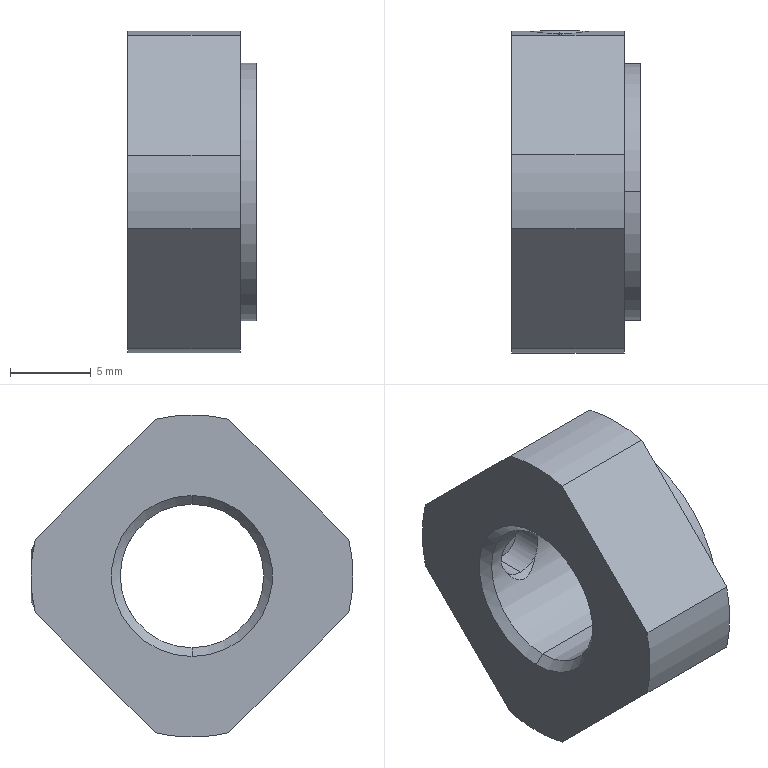Part | STEP file | Mirror BNR10 | 2 solids | 49 faces | box 8 x 20 x 20 mm | volume 1587 mm3 | cone 20 | plane 16 | cylinder 13 | commonest cylinder face diameters 20 x5 3.242 x2 4 x2 8.917 x2 16 x2
STEP:
#1=CARTESIAN_POINT('',(7.,0.,-10.));
#2=VERTEX_POINT('',#1);
#3=CARTESIAN_POINT('',(7.,2.285,-9.735));
#4=VERTEX_POINT('',#3);
#5=CARTESIAN_POINT('',(7.,0.,0.));
#6=DIRECTION('',(1.,0.,0.));
#7=DIRECTION('',(0.,0.,-1.));
#8=AXIS2_PLACEMENT_3D('',#5,#6,#7);
#9=CIRCLE('',#8,10.);
#10=EDGE_CURVE('',#2,#4,#9,.T.);
#11=ORIENTED_EDGE('',*,*,#10,.F.);
#12=CARTESIAN_POINT('',(0.,0.,-10.));
#13=VERTEX_POINT('',#12);
#14=CARTESIAN_POINT('',(8.,0.,-10.));
#15=DIRECTION('',(-1.,0.,0.));
#16=VECTOR('',#15,1000.);
#17=LINE('',#14,#16);
#18=EDGE_CURVE('',#2,#13,#17,.T.);
#19=ORIENTED_EDGE('',*,*,#18,.T.);
#20=CARTESIAN_POINT('',(0.,2.285,-9.735));
#21=VERTEX_POINT('',#20);
#22=CARTESIAN_POINT('',(0.,0.,0.));
#23=DIRECTION('',(1.,0.,0.));
#24=DIRECTION('',(0.,0.,-1.));
#25=AXIS2_PLACEMENT_3D('',#22,#23,#24);
#26=CIRCLE('',#25,10.);
#27=EDGE_CURVE('',#13,#21,#26,.T.);
#28=ORIENTED_EDGE('',*,*,#27,.T.);
#29=CARTESIAN_POINT('',(8.,2.285,-9.735));
#30=DIRECTION('',(-1.,0.,0.));
#31=VECTOR('',#30,1000.);
#32=LINE('',#29,#31);
#33=EDGE_CURVE('',#4,#21,#32,.T.);
#34=ORIENTED_EDGE('',*,*,#33,.F.);
#35=EDGE_LOOP('',(#11,#19,#28,#34));
#36=FACE_OUTER_BOUND('',#35,.T.);
#37=CARTESIAN_POINT('',(8.,0.,0.));
#38=DIRECTION('',(-1.,0.,0.));
#39=DIRECTION('',(0.,0.,-1.));
#40=AXIS2_PLACEMENT_3D('',#37,#38,#39);
#41=CYLINDRICAL_SURFACE('',#40,10.);
#42=ADVANCED_FACE('',(#36),#41,.T.);
#43=CARTESIAN_POINT('',(0.5415,0.,-4.458));
#44=VERTEX_POINT('',#43);
#45=CARTESIAN_POINT('',(0.5415,0.,4.458));
#46=VERTEX_POINT('',#45);
#47=CARTESIAN_POINT('',(0.5415,0.,0.));
#48=DIRECTION('',(1.,0.,0.));
#49=DIRECTION('',(0.,0.,-1.));
#50=AXIS2_PLACEMENT_3D('',#47,#48,#49);
#51=CIRCLE('',#50,4.458);
#52=EDGE_CURVE('',#44,#46,#51,.T.);
#53=ORIENTED_EDGE('',*,*,#52,.T.);
#54=CARTESIAN_POINT('',(0.,0.,5.));
#55=VERTEX_POINT('',#54);
#56=CARTESIAN_POINT('',(0.,0.,5.));
#57=DIRECTION('',(-0.7071,0.,0.7071));
#58=VECTOR('',#57,1000.);
#59=LINE('',#56,#58);
#60=EDGE_CURVE('',#46,#55,#59,.T.);
#61=ORIENTED_EDGE('',*,*,#60,.T.);
#62=CARTESIAN_POINT('',(0.,0.,-5.));
#63=VERTEX_POINT('',#62);
#64=CARTESIAN_POINT('',(0.,0.,0.));
#65=DIRECTION('',(-1.,0.,0.));
#66=DIRECTION('',(0.,0.,-1.));
#67=AXIS2_PLACEMENT_3D('',#64,#65,#66);
#68=CIRCLE('',#67,5.);
#69=EDGE_CURVE('',#55,#63,#68,.T.);
#70=ORIENTED_EDGE('',*,*,#69,.T.);
#71=CARTESIAN_POINT('',(0.,0.,-5.));
#72=DIRECTION('',(-0.7071,0.,-0.7071));
#73=VECTOR('',#72,1000.);
#74=LINE('',#71,#73);
#75=EDGE_CURVE('',#44,#63,#74,.T.);
#76=ORIENTED_EDGE('',*,*,#75,.F.);
#77=EDGE_LOOP('',(#53,#61,#70,#76));
#78=FACE_OUTER_BOUND('',#77,.T.);
#79=CARTESIAN_POINT('',(0.,0.,0.));
#80=DIRECTION('',(-1.,0.,0.));
#81=DIRECTION('',(0.,0.,-1.));
#82=AXIS2_PLACEMENT_3D('',#79,#80,#81);
#83=CONICAL_SURFACE('',#82,5.,0.7854);
#84=ADVANCED_FACE('',(#78),#83,.F.);
#85=CARTESIAN_POINT('',(3.,9.621,-1.621));
#86=VERTEX_POINT('',#85);
#87=CARTESIAN_POINT('',(3.,9.621,1.621));
#88=VERTEX_POINT('',#87);
#89=CARTESIAN_POINT('',(3.,9.621,0.));
#90=DIRECTION('',(0.,-1.,0.));
#91=DIRECTION('',(0.,0.,-1.));
#92=AXIS2_PLACEMENT_3D('',#89,#90,#91);
#93=CIRCLE('',#92,1.621);
#94=EDGE_CURVE('',#86,#88,#93,.T.);
#95=ORIENTED_EDGE('',*,*,#94,.T.);
#96=CARTESIAN_POINT('',(3.,9.831,1.831));
#97=VERTEX_POINT('',#96);
#98=CARTESIAN_POINT('',(3.,10.004,2.004));
#99=DIRECTION('',(0.,0.7071,0.7071));
#100=VECTOR('',#99,1000.);
#101=LINE('',#98,#100);
#102=EDGE_CURVE('',#88,#97,#101,.T.);
#103=ORIENTED_EDGE('',*,*,#102,.T.);
#104=CARTESIAN_POINT('',(3.,9.831,-1.831));
#105=VERTEX_POINT('',#104);
#106=CARTESIAN_POINT('',(3.,9.831,1.831));
#107=CARTESIAN_POINT('',(3.126,9.831,1.831));
#108=CARTESIAN_POINT('',(3.251,9.833,1.82));
#109=CARTESIAN_POINT('',(3.497,9.841,1.777));
#110=CARTESIAN_POINT('',(3.619,9.847,1.744));
#111=CARTESIAN_POINT('',(3.856,9.862,1.658));
#112=CARTESIAN_POINT('',(3.968,9.871,1.605));
#113=CARTESIAN_POINT('',(4.183,9.89,1.479));
#114=CARTESIAN_POINT('',(4.286,9.901,1.405));
#115=CARTESIAN_POINT('',(4.475,9.923,1.24));
#116=CARTESIAN_POINT('',(4.56,9.934,1.15));
#117=CARTESIAN_POINT('',(4.712,9.955,0.9524));
#118=CARTESIAN_POINT('',(4.779,9.965,0.8438));
#119=CARTESIAN_POINT('',(4.887,9.982,0.6182));
#120=CARTESIAN_POINT('',(4.928,9.988,0.5007));
#121=CARTESIAN_POINT('',(4.985,9.997,0.2558));
#122=CARTESIAN_POINT('',(5.,10.,0.1289));
#123=CARTESIAN_POINT('',(5.,10.,-0.1212));
#124=CARTESIAN_POINT('',(4.986,9.998,-0.2475));
#125=CARTESIAN_POINT('',(4.93,9.989,-0.4936));
#126=CARTESIAN_POINT('',(4.889,9.982,-0.6117));
#127=CARTESIAN_POINT('',(4.728,9.957,-0.9525));
#128=CARTESIAN_POINT('',(4.572,9.934,-1.155));
#129=CARTESIAN_POINT('',(4.288,9.901,-1.404));
#130=CARTESIAN_POINT('',(4.187,9.891,-1.477));
#131=CARTESIAN_POINT('',(3.971,9.871,-1.604));
#132=CARTESIAN_POINT('',(3.856,9.862,-1.658));
#133=CARTESIAN_POINT('',(3.62,9.847,-1.744));
#134=CARTESIAN_POINT('',(3.5,9.841,-1.776));
#135=CARTESIAN_POINT('',(3.252,9.833,-1.82));
#136=CARTESIAN_POINT('',(3.125,9.831,-1.831));
#137=CARTESIAN_POINT('',(3.,9.831,-1.831));
#138=B_SPLINE_CURVE_WITH_KNOTS('',3,(#106,#107,#108,#109,#110,#111,#112,#113,#114,#115,#116,#117,#118,#119,#120,#121,#122,#123,#124,#125,#126,#127,#128,#129,#130,#131,#132,#133,#134,#135,#136,#137),.UNSPECIFIED.,.F.,.F.,(4,2,2,2,2,2,2,2,2,2,2,2,2,2,2,4),(0.003101,0.003476,0.00385,0.004225,0.0046,0.004974,0.005349,0.005723,0.006098,0.006473,0.006847,0.007597,0.007971,0.008346,0.00872,0.009095),.UNSPECIFIED.);
#139=EDGE_CURVE('',#97,#105,#138,.T.);
#140=ORIENTED_EDGE('',*,*,#139,.T.);
#141=CARTESIAN_POINT('',(3.,10.004,-2.004));
#142=DIRECTION('',(0.,0.7071,-0.7071));
#143=VECTOR('',#142,1000.);
#144=LINE('',#141,#143);
#145=EDGE_CURVE('',#86,#105,#144,.T.);
#146=ORIENTED_EDGE('',*,*,#145,.F.);
#147=EDGE_LOOP('',(#95,#103,#140,#146));
#148=FACE_OUTER_BOUND('',#147,.T.);
#149=CARTESIAN_POINT('',(3.,10.004,0.));
#150=DIRECTION('',(0.,1.,0.));
#151=DIRECTION('',(0.,0.,-1.));
#152=AXIS2_PLACEMENT_3D('',#149,#150,#151);
#153=CONICAL_SURFACE('',#152,2.004,0.7854);
#154=ADVANCED_FACE('',(#148),#153,.F.);
#155=CARTESIAN_POINT('',(1.75,4.337,-1.032));
#156=VERTEX_POINT('',#155);
#157=CARTESIAN_POINT('',(1.75,4.338,1.032));
#158=VERTEX_POINT('',#157);
#159=CARTESIAN_POINT('',(1.75,4.337,-1.032));
#160=CARTESIAN_POINT('',(1.631,4.372,-0.888));
#161=CARTESIAN_POINT('',(1.539,4.402,-0.7274));
#162=CARTESIAN_POINT('',(1.412,4.446,-0.3743));
#163=CARTESIAN_POINT('',(1.379,4.458,-0.1893));
#164=CARTESIAN_POINT('',(1.379,4.459,0.1881));
#165=CARTESIAN_POINT('',(1.412,4.446,0.3743));
#166=CARTESIAN_POINT('',(1.539,4.403,0.7258));
#167=CARTESIAN_POINT('',(1.631,4.372,0.888));
#168=CARTESIAN_POINT('',(1.75,4.338,1.032));
#169=B_SPLINE_CURVE_WITH_KNOTS('',3,(#159,#160,#161,#162,#163,#164,#165,#166,#167,#168),.UNSPECIFIED.,.F.,.F.,(4,2,2,2,4),(0.,0.0005603,0.001121,0.001681,0.002241),.UNSPECIFIED.);
#170=EDGE_CURVE('',#156,#158,#169,.T.);
#171=ORIENTED_EDGE('',*,*,#170,.T.);
#172=CARTESIAN_POINT('',(3.,4.01,1.948));
#173=VERTEX_POINT('',#172);
#174=CARTESIAN_POINT('',(1.75,4.338,1.032));
#175=CARTESIAN_POINT('',(1.812,4.309,1.153));
#176=CARTESIAN_POINT('',(1.885,4.276,1.266));
#177=CARTESIAN_POINT('',(2.05,4.209,1.475));
#178=CARTESIAN_POINT('',(2.144,4.173,1.572));
#179=CARTESIAN_POINT('',(2.354,4.105,1.742));
#180=CARTESIAN_POINT('',(2.469,4.073,1.814));
#181=CARTESIAN_POINT('',(2.723,4.025,1.918));
#182=CARTESIAN_POINT('',(2.862,4.01,1.948));
#183=CARTESIAN_POINT('',(3.,4.01,1.948));
#184=B_SPLINE_CURVE_WITH_KNOTS('',3,(#174,#175,#176,#177,#178,#179,#180,#181,#182,#183),.UNSPECIFIED.,.F.,.F.,(4,2,2,2,4),(0.,0.0004125,0.0008251,0.001238,0.00165),.UNSPECIFIED.);
#185=EDGE_CURVE('',#158,#173,#184,.T.);
#186=ORIENTED_EDGE('',*,*,#185,.T.);
#187=CARTESIAN_POINT('',(4.25,4.337,1.032));
#188=VERTEX_POINT('',#187);
#189=CARTESIAN_POINT('',(3.,4.01,1.948));
#190=CARTESIAN_POINT('',(3.138,4.01,1.948));
#191=CARTESIAN_POINT('',(3.277,4.025,1.918));
#192=CARTESIAN_POINT('',(3.53,4.073,1.814));
#193=CARTESIAN_POINT('',(3.646,4.105,1.742));
#194=CARTESIAN_POINT('',(3.855,4.173,1.573));
#195=CARTESIAN_POINT('',(3.949,4.209,1.476));
#196=CARTESIAN_POINT('',(4.115,4.276,1.266));
#197=CARTESIAN_POINT('',(4.188,4.309,1.153));
#198=CARTESIAN_POINT('',(4.25,4.337,1.032));
#199=B_SPLINE_CURVE_WITH_KNOTS('',3,(#189,#190,#191,#192,#193,#194,#195,#196,#197,#198),.UNSPECIFIED.,.F.,.F.,(4,2,2,2,4),(0.00165,0.002062,0.002474,0.002887,0.003299),.UNSPECIFIED.);
#200=EDGE_CURVE('',#173,#188,#199,.T.);
#201=ORIENTED_EDGE('',*,*,#200,.T.);
#202=CARTESIAN_POINT('',(4.25,4.338,-1.032));
#203=VERTEX_POINT('',#202);
#204=CARTESIAN_POINT('',(4.25,4.337,1.032));
#205=CARTESIAN_POINT('',(4.369,4.372,0.888));
#206=CARTESIAN_POINT('',(4.461,4.402,0.7274));
#207=CARTESIAN_POINT('',(4.588,4.446,0.3743));
#208=CARTESIAN_POINT('',(4.621,4.458,0.1893));
#209=CARTESIAN_POINT('',(4.621,4.459,-0.1881));
#210=CARTESIAN_POINT('',(4.588,4.446,-0.3743));
#211=CARTESIAN_POINT('',(4.461,4.403,-0.7258));
#212=CARTESIAN_POINT('',(4.369,4.372,-0.888));
#213=CARTESIAN_POINT('',(4.25,4.338,-1.032));
#214=B_SPLINE_CURVE_WITH_KNOTS('',3,(#204,#205,#206,#207,#208,#209,#210,#211,#212,#213),.UNSPECIFIED.,.F.,.F.,(4,2,2,2,4),(0.,0.0005603,0.001121,0.001681,0.002241),.UNSPECIFIED.);
#215=EDGE_CURVE('',#188,#203,#214,.T.);
#216=ORIENTED_EDGE('',*,*,#215,.T.);
#217=CARTESIAN_POINT('',(4.25,4.338,-1.032));
#218=CARTESIAN_POINT('',(4.188,4.309,-1.153));
#219=CARTESIAN_POINT('',(4.115,4.276,-1.266));
#220=CARTESIAN_POINT('',(3.95,4.209,-1.475));
#221=CARTESIAN_POINT('',(3.856,4.173,-1.572));
#222=CARTESIAN_POINT('',(3.647,4.105,-1.742));
#223=CARTESIAN_POINT('',(3.531,4.073,-1.814));
#224=CARTESIAN_POINT('',(3.277,4.025,-1.918));
#225=CARTESIAN_POINT('',(3.139,4.01,-1.948));
#226=CARTESIAN_POINT('',(2.863,4.01,-1.948));
#227=CARTESIAN_POINT('',(2.724,4.025,-1.918));
#228=CARTESIAN_POINT('',(2.47,4.073,-1.815));
#229=CARTESIAN_POINT('',(2.354,4.105,-1.742));
#230=CARTESIAN_POINT('',(2.146,4.173,-1.574));
#231=CARTESIAN_POINT('',(2.051,4.209,-1.476));
#232=CARTESIAN_POINT('',(1.885,4.276,-1.266));
#233=CARTESIAN_POINT('',(1.812,4.309,-1.153));
#234=CARTESIAN_POINT('',(1.75,4.337,-1.032));
#235=B_SPLINE_CURVE_WITH_KNOTS('',3,(#217,#218,#219,#220,#221,#222,#223,#224,#225,#226,#227,#228,#229,#230,#231,#232,#233,#234),.UNSPECIFIED.,.F.,.F.,(4,2,2,2,2,2,2,2,4),(0.,0.0004123,0.0008247,0.001237,0.001649,0.002062,0.002474,0.002886,0.003299),.UNSPECIFIED.);
#236=EDGE_CURVE('',#203,#156,#235,.T.);
#237=ORIENTED_EDGE('',*,*,#236,.T.);
#238=EDGE_LOOP('',(#171,#186,#201,#216,#237));
#239=FACE_BOUND('',#238,.T.);
#240=CARTESIAN_POINT('',(7.458,0.,-4.458));
#241=VERTEX_POINT('',#240);
#242=CARTESIAN_POINT('',(7.458,0.,4.458));
#243=VERTEX_POINT('',#242);
#244=CARTESIAN_POINT('',(7.458,0.,0.));
#245=DIRECTION('',(1.,0.,0.));
#246=DIRECTION('',(0.,0.,-1.));
#247=AXIS2_PLACEMENT_3D('',#244,#245,#246);
#248=CIRCLE('',#247,4.458);
#249=EDGE_CURVE('',#241,#243,#248,.T.);
#250=ORIENTED_EDGE('',*,*,#249,.T.);
#251=CARTESIAN_POINT('',(8.,0.,4.458));
#252=DIRECTION('',(-1.,0.,0.));
#253=VECTOR('',#252,1000.);
#254=LINE('',#251,#253);
#255=EDGE_CURVE('',#243,#46,#254,.T.);
#256=ORIENTED_EDGE('',*,*,#255,.T.);
#257=ORIENTED_EDGE('',*,*,#52,.F.);
#258=CARTESIAN_POINT('',(8.,0.,-4.458));
#259=DIRECTION('',(-1.,0.,0.));
#260=VECTOR('',#259,1000.);
#261=LINE('',#258,#260);
#262=EDGE_CURVE('',#241,#44,#261,.T.);
#263=ORIENTED_EDGE('',*,*,#262,.F.);
#264=EDGE_LOOP('',(#250,#256,#257,#263));
#265=FACE_OUTER_BOUND('',#264,.T.);
#266=CARTESIAN_POINT('',(8.,0.,0.));
#267=DIRECTION('',(-1.,0.,0.));
#268=DIRECTION('',(0.,0.,-1.));
#269=AXIS2_PLACEMENT_3D('',#266,#267,#268);
#270=CYLINDRICAL_SURFACE('',#269,4.458);
#271=ADVANCED_FACE('',(#239,#265),#270,.F.);
#272=CARTESIAN_POINT('',(8.,0.,8.));
#273=VERTEX_POINT('',#272);
#274=CARTESIAN_POINT('',(8.,0.,-8.));
#275=VERTEX_POINT('',#274);
#276=CARTESIAN_POINT('',(8.,0.,0.));
#277=DIRECTION('',(1.,0.,0.));
#278=DIRECTION('',(0.,0.,-1.));
#279=AXIS2_PLACEMENT_3D('',#276,#277,#278);
#280=CIRCLE('',#279,8.);
#281=EDGE_CURVE('',#273,#275,#280,.T.);
#282=ORIENTED_EDGE('',*,*,#281,.F.);
#283=CARTESIAN_POINT('',(7.,0.,8.));
#284=VERTEX_POINT('',#283);
#285=CARTESIAN_POINT('',(8.,0.,8.));
#286=DIRECTION('',(-1.,0.,0.));
#287=VECTOR('',#286,1000.);
#288=LINE('',#285,#287);
#289=EDGE_CURVE('',#273,#284,#288,.T.);
#290=ORIENTED_EDGE('',*,*,#289,.T.);
#291=CARTESIAN_POINT('',(7.,0.,-8.));
#292=VERTEX_POINT('',#291);
#293=CARTESIAN_POINT('',(7.,0.,0.));
#294=DIRECTION('',(1.,0.,0.));
#295=DIRECTION('',(0.,0.,-1.));
#296=AXIS2_PLACEMENT_3D('',#293,#294,#295);
#297=CIRCLE('',#296,8.);
#298=EDGE_CURVE('',#284,#292,#297,.T.);
#299=ORIENTED_EDGE('',*,*,#298,.T.);
#300=CARTESIAN_POINT('',(8.,0.,-8.));
#301=DIRECTION('',(-1.,0.,0.));
#302=VECTOR('',#301,1000.);
#303=LINE('',#300,#302);
#304=EDGE_CURVE('',#275,#292,#303,.T.);
#305=ORIENTED_EDGE('',*,*,#304,.F.);
#306=EDGE_LOOP('',(#282,#290,#299,#305));
#307=FACE_OUTER_BOUND('',#306,.T.);
#308=CARTESIAN_POINT('',(8.,0.,0.));
#309=DIRECTION('',(-1.,0.,0.));
#310=DIRECTION('',(0.,0.,-1.));
#311=AXIS2_PLACEMENT_3D('',#308,#309,#310);
#312=CYLINDRICAL_SURFACE('',#311,8.);
#313=ADVANCED_FACE('',(#307),#312,.T.);
#314=CARTESIAN_POINT('',(3.,4.338,1.621));
#315=VERTEX_POINT('',#314);
#316=CARTESIAN_POINT('',(3.,4.338,0.));
#317=DIRECTION('',(0.,-1.,0.));
#318=DIRECTION('',(0.,0.,-1.));
#319=AXIS2_PLACEMENT_3D('',#316,#317,#318);
#320=CIRCLE('',#319,1.621);
#321=EDGE_CURVE('',#188,#315,#320,.T.);
#322=ORIENTED_EDGE('',*,*,#321,.T.);
#323=CARTESIAN_POINT('',(3.,3.959,1.621));
#324=DIRECTION('',(0.,1.,0.));
#325=VECTOR('',#324,1000.);
#326=LINE('',#323,#325);
#327=EDGE_CURVE('',#315,#88,#326,.T.);
#328=ORIENTED_EDGE('',*,*,#327,.T.);
#329=ORIENTED_EDGE('',*,*,#94,.F.);
#330=CARTESIAN_POINT('',(3.,4.338,-1.621));
#331=VERTEX_POINT('',#330);
#332=CARTESIAN_POINT('',(3.,3.959,-1.621));
#333=DIRECTION('',(0.,1.,0.));
#334=VECTOR('',#333,1000.);
#335=LINE('',#332,#334);
#336=EDGE_CURVE('',#331,#86,#335,.T.);
#337=ORIENTED_EDGE('',*,*,#336,.F.);
#338=CARTESIAN_POINT('',(3.,4.338,0.));
#339=DIRECTION('',(0.,-1.,0.));
#340=DIRECTION('',(0.,0.,-1.));
#341=AXIS2_PLACEMENT_3D('',#338,#339,#340);
#342=CIRCLE('',#341,1.621);
#343=EDGE_CURVE('',#331,#203,#342,.T.);
#344=ORIENTED_EDGE('',*,*,#343,.T.);
#345=ORIENTED_EDGE('',*,*,#215,.F.);
#346=EDGE_LOOP('',(#322,#328,#329,#337,#344,#345));
#347=FACE_OUTER_BOUND('',#346,.T.);
#348=CARTESIAN_POINT('',(3.,3.959,0.));
#349=DIRECTION('',(0.,1.,0.));
#350=DIRECTION('',(0.,0.,-1.));
#351=AXIS2_PLACEMENT_3D('',#348,#349,#350);
#352=CYLINDRICAL_SURFACE('',#351,1.621);
#353=ADVANCED_FACE('',(#347),#352,.F.);
#354=CARTESIAN_POINT('',(3.,4.338,0.));
#355=DIRECTION('',(0.,-1.,0.));
#356=DIRECTION('',(0.,0.,-1.));
#357=AXIS2_PLACEMENT_3D('',#354,#355,#356);
#358=CIRCLE('',#357,1.621);
#359=EDGE_CURVE('',#315,#158,#358,.T.);
#360=ORIENTED_EDGE('',*,*,#359,.F.);
#361=CARTESIAN_POINT('',(3.,4.008,1.95));
#362=DIRECTION('',(0.,-0.7071,0.7071));
#363=VECTOR('',#362,1000.);
#364=LINE('',#361,#363);
#365=EDGE_CURVE('',#315,#173,#364,.T.);
#366=ORIENTED_EDGE('',*,*,#365,.T.);
#367=ORIENTED_EDGE('',*,*,#185,.F.);
#368=EDGE_LOOP('',(#360,#366,#367));
#369=FACE_OUTER_BOUND('',#368,.T.);
#370=CARTESIAN_POINT('',(3.,4.008,0.));
#371=DIRECTION('',(0.,-1.,0.));
#372=DIRECTION('',(0.,0.,1.));
#373=AXIS2_PLACEMENT_3D('',#370,#371,#372);
#374=CONICAL_SURFACE('',#373,1.95,0.7854);
#375=ADVANCED_FACE('',(#369),#374,.F.);
#376=ORIENTED_EDGE('',*,*,#249,.F.);
#377=CARTESIAN_POINT('',(8.,0.,-5.));
#378=VERTEX_POINT('',#377);
#379=CARTESIAN_POINT('',(8.,0.,-5.));
#380=DIRECTION('',(0.7071,0.,-0.7071));
#381=VECTOR('',#380,1000.);
#382=LINE('',#379,#381);
#383=EDGE_CURVE('',#241,#378,#382,.T.);
#384=ORIENTED_EDGE('',*,*,#383,.T.);
#385=CARTESIAN_POINT('',(8.,0.,5.));
#386=VERTEX_POINT('',#385);
#387=CARTESIAN_POINT('',(8.,0.,0.));
#388=DIRECTION('',(1.,0.,0.));
#389=DIRECTION('',(0.,0.,1.));
#390=AXIS2_PLACEMENT_3D('',#387,#388,#389);
#391=CIRCLE('',#390,5.);
#392=EDGE_CURVE('',#378,#386,#391,.T.);
#393=ORIENTED_EDGE('',*,*,#392,.T.);
#394=CARTESIAN_POINT('',(8.,0.,5.));
#395=DIRECTION('',(0.7071,0.,0.7071));
#396=VECTOR('',#395,1000.);
#397=LINE('',#394,#396);
#398=EDGE_CURVE('',#243,#386,#397,.T.);
#399=ORIENTED_EDGE('',*,*,#398,.F.);
#400=EDGE_LOOP('',(#376,#384,#393,#399));
#401=FACE_OUTER_BOUND('',#400,.T.);
#402=CARTESIAN_POINT('',(8.,0.,0.));
#403=DIRECTION('',(1.,0.,0.));
#404=DIRECTION('',(0.,0.,1.));
#405=AXIS2_PLACEMENT_3D('',#402,#403,#404);
#406=CONICAL_SURFACE('',#405,5.,0.7854);
#407=ADVANCED_FACE('',(#401),#406,.F.);
#408=CARTESIAN_POINT('',(8.,0.,0.));
#409=DIRECTION('',(1.,0.,0.));
#410=DIRECTION('',(0.,0.,1.));
#411=AXIS2_PLACEMENT_3D('',#408,#409,#410);
#412=CIRCLE('',#411,5.);
#413=EDGE_CURVE('',#386,#378,#412,.T.);
#414=ORIENTED_EDGE('',*,*,#413,.F.);
#415=ORIENTED_EDGE('',*,*,#392,.F.);
#416=EDGE_LOOP('',(#414,#415));
#417=FACE_BOUND('',#416,.T.);
#418=CARTESIAN_POINT('',(8.,0.,0.));
#419=DIRECTION('',(1.,0.,0.));
#420=DIRECTION('',(0.,0.,-1.));
#421=AXIS2_PLACEMENT_3D('',#418,#419,#420);
#422=CIRCLE('',#421,8.);
#423=EDGE_CURVE('',#275,#273,#422,.T.);
#424=ORIENTED_EDGE('',*,*,#423,.T.);
#425=ORIENTED_EDGE('',*,*,#281,.T.);
#426=EDGE_LOOP('',(#424,#425));
#427=FACE_OUTER_BOUND('',#426,.T.);
#428=CARTESIAN_POINT('',(8.,5.,0.));
#429=DIRECTION('',(1.,0.,0.));
#430=DIRECTION('',(0.,0.,1.));
#431=AXIS2_PLACEMENT_3D('',#428,#429,#430);
#432=PLANE('',#431);
#433=ADVANCED_FACE('',(#417,#427),#432,.T.);
#434=ORIENTED_EDGE('',*,*,#383,.F.);
#435=CARTESIAN_POINT('',(7.458,0.,0.));
#436=DIRECTION('',(1.,0.,0.));
#437=DIRECTION('',(0.,0.,-1.));
#438=AXIS2_PLACEMENT_3D('',#435,#436,#437);
#439=CIRCLE('',#438,4.458);
#440=EDGE_CURVE('',#243,#241,#439,.T.);
#441=ORIENTED_EDGE('',*,*,#440,.F.);
#442=ORIENTED_EDGE('',*,*,#398,.T.);
#443=ORIENTED_EDGE('',*,*,#413,.T.);
#444=EDGE_LOOP('',(#434,#441,#442,#443));
#445=FACE_OUTER_BOUND('',#444,.T.);
#446=CARTESIAN_POINT('',(8.,0.,0.));
#447=DIRECTION('',(1.,0.,0.));
#448=DIRECTION('',(0.,0.,1.));
#449=AXIS2_PLACEMENT_3D('',#446,#447,#448);
#450=CONICAL_SURFACE('',#449,5.,0.7854);
#451=ADVANCED_FACE('',(#445),#450,.F.);
#452=ORIENTED_EDGE('',*,*,#236,.F.);
#453=ORIENTED_EDGE('',*,*,#343,.F.);
#454=CARTESIAN_POINT('',(3.,4.338,0.));
#455=DIRECTION('',(0.,-1.,0.));
#456=DIRECTION('',(0.,0.,-1.));
#457=AXIS2_PLACEMENT_3D('',#454,#455,#456);
#458=CIRCLE('',#457,1.621);
#459=EDGE_CURVE('',#156,#331,#458,.T.);
#460=ORIENTED_EDGE('',*,*,#459,.F.);
#461=EDGE_LOOP('',(#452,#453,#460));
#462=FACE_OUTER_BOUND('',#461,.T.);
#463=CARTESIAN_POINT('',(3.,4.008,0.));
#464=DIRECTION('',(0.,-1.,0.));
#465=DIRECTION('',(0.,0.,1.));
#466=AXIS2_PLACEMENT_3D('',#463,#464,#465);
#467=CONICAL_SURFACE('',#466,1.95,0.7854);
#468=ADVANCED_FACE('',(#462),#467,.F.);
#469=ORIENTED_EDGE('',*,*,#365,.F.);
#470=ORIENTED_EDGE('',*,*,#321,.F.);
#471=ORIENTED_EDGE('',*,*,#200,.F.);
#472=EDGE_LOOP('',(#469,#470,#471));
#473=FACE_OUTER_BOUND('',#472,.T.);
#474=CARTESIAN_POINT('',(3.,4.008,0.));
#475=DIRECTION('',(0.,-1.,0.));
#476=DIRECTION('',(0.,0.,1.));
#477=AXIS2_PLACEMENT_3D('',#474,#475,#476);
#478=CONICAL_SURFACE('',#477,1.95,0.7854);
#479=ADVANCED_FACE('',(#473),#478,.F.);
#480=ORIENTED_EDGE('',*,*,#327,.F.);
#481=ORIENTED_EDGE('',*,*,#359,.T.);
#482=ORIENTED_EDGE('',*,*,#170,.F.);
#483=ORIENTED_EDGE('',*,*,#459,.T.);
#484=ORIENTED_EDGE('',*,*,#336,.T.);
#485=CARTESIAN_POINT('',(3.,9.621,0.));
#486=DIRECTION('',(0.,-1.,0.));
#487=DIRECTION('',(0.,0.,-1.));
#488=AXIS2_PLACEMENT_3D('',#485,#486,#487);
#489=CIRCLE('',#488,1.621);
#490=EDGE_CURVE('',#88,#86,#489,.T.);
#491=ORIENTED_EDGE('',*,*,#490,.F.);
#492=EDGE_LOOP('',(#480,#481,#482,#483,#484,#491));
#493=FACE_OUTER_BOUND('',#492,.T.);
#494=CARTESIAN_POINT('',(3.,3.959,0.));
#495=DIRECTION('',(0.,1.,0.));
#496=DIRECTION('',(0.,0.,-1.));
#497=AXIS2_PLACEMENT_3D('',#494,#495,#496);
#498=CYLINDRICAL_SURFACE('',#497,1.621);
#499=ADVANCED_FACE('',(#493),#498,.F.);
#500=ORIENTED_EDGE('',*,*,#289,.F.);
#501=ORIENTED_EDGE('',*,*,#423,.F.);
#502=ORIENTED_EDGE('',*,*,#304,.T.);
#503=CARTESIAN_POINT('',(7.,0.,0.));
#504=DIRECTION('',(1.,0.,0.));
#505=DIRECTION('',(0.,0.,-1.));
#506=AXIS2_PLACEMENT_3D('',#503,#504,#505);
#507=CIRCLE('',#506,8.);
#508=EDGE_CURVE('',#292,#284,#507,.T.);
#509=ORIENTED_EDGE('',*,*,#508,.T.);
#510=EDGE_LOOP('',(#500,#501,#502,#509));
#511=FACE_OUTER_BOUND('',#510,.T.);
#512=CARTESIAN_POINT('',(8.,0.,0.));
#513=DIRECTION('',(-1.,0.,0.));
#514=DIRECTION('',(0.,0.,-1.));
#515=AXIS2_PLACEMENT_3D('',#512,#513,#514);
#516=CYLINDRICAL_SURFACE('',#515,8.);
#517=ADVANCED_FACE('',(#511),#516,.T.);
#518=ORIENTED_EDGE('',*,*,#255,.F.);
#519=ORIENTED_EDGE('',*,*,#440,.T.);
#520=ORIENTED_EDGE('',*,*,#262,.T.);
#521=CARTESIAN_POINT('',(0.5415,0.,0.));
#522=DIRECTION('',(1.,0.,0.));
#523=DIRECTION('',(0.,0.,-1.));
#524=AXIS2_PLACEMENT_3D('',#521,#522,#523);
#525=CIRCLE('',#524,4.458);
#526=EDGE_CURVE('',#46,#44,#525,.T.);
#527=ORIENTED_EDGE('',*,*,#526,.F.);
#528=EDGE_LOOP('',(#518,#519,#520,#527));
#529=FACE_OUTER_BOUND('',#528,.T.);
#530=CARTESIAN_POINT('',(8.,0.,0.));
#531=DIRECTION('',(-1.,0.,0.));
#532=DIRECTION('',(0.,0.,-1.));
#533=AXIS2_PLACEMENT_3D('',#530,#531,#532);
#534=CYLINDRICAL_SURFACE('',#533,4.458);
#535=ADVANCED_FACE('',(#529),#534,.F.);
#536=ORIENTED_EDGE('',*,*,#102,.F.);
#537=ORIENTED_EDGE('',*,*,#490,.T.);
#538=ORIENTED_EDGE('',*,*,#145,.T.);
#539=CARTESIAN_POINT('',(3.,9.831,-1.831));
#540=CARTESIAN_POINT('',(2.75,9.831,-1.831));
#541=CARTESIAN_POINT('',(2.497,9.839,-1.787));
#542=CARTESIAN_POINT('',(2.028,9.869,-1.616));
#543=CARTESIAN_POINT('',(1.807,9.89,-1.487));
#544=CARTESIAN_POINT('',(1.432,9.934,-1.159));
#545=CARTESIAN_POINT('',(1.275,9.957,-0.9559));
#546=CARTESIAN_POINT('',(1.06,9.99,-0.5063));
#547=CARTESIAN_POINT('',(1.,10.,-0.2512));
#548=CARTESIAN_POINT('',(1.,10.,0.1259));
#549=CARTESIAN_POINT('',(1.014,9.998,0.2499));
#550=CARTESIAN_POINT('',(1.07,9.989,0.4946));
#551=CARTESIAN_POINT('',(1.112,9.982,0.615));
#552=CARTESIAN_POINT('',(1.219,9.965,0.8408));
#553=CARTESIAN_POINT('',(1.286,9.955,0.9487));
#554=CARTESIAN_POINT('',(1.438,9.934,1.148));
#555=CARTESIAN_POINT('',(1.524,9.923,1.239));
#556=CARTESIAN_POINT('',(1.712,9.901,1.404));
#557=CARTESIAN_POINT('',(1.815,9.89,1.478));
#558=CARTESIAN_POINT('',(2.03,9.871,1.605));
#559=CARTESIAN_POINT('',(2.144,9.862,1.658));
#560=CARTESIAN_POINT('',(2.499,9.839,1.788));
#561=CARTESIAN_POINT('',(2.747,9.831,1.831));
#562=CARTESIAN_POINT('',(3.,9.831,1.831));
#563=B_SPLINE_CURVE_WITH_KNOTS('',3,(#539,#540,#541,#542,#543,#544,#545,#546,#547,#548,#549,#550,#551,#552,#553,#554,#555,#556,#557,#558,#559,#560,#561,#562),.UNSPECIFIED.,.F.,.F.,(4,2,2,2,2,2,2,2,2,2,2,4),(0.009095,0.009844,0.01059,0.01134,0.01209,0.01247,0.01284,0.01321,0.01359,0.01396,0.01434,0.01509),.UNSPECIFIED.);
#564=EDGE_CURVE('',#105,#97,#563,.T.);
#565=ORIENTED_EDGE('',*,*,#564,.T.);
#566=EDGE_LOOP('',(#536,#537,#538,#565));
#567=FACE_OUTER_BOUND('',#566,.T.);
#568=CARTESIAN_POINT('',(3.,10.004,0.));
#569=DIRECTION('',(0.,1.,0.));
#570=DIRECTION('',(0.,0.,-1.));
#571=AXIS2_PLACEMENT_3D('',#568,#569,#570);
#572=CONICAL_SURFACE('',#571,2.004,0.7854);
#573=ADVANCED_FACE('',(#567),#572,.F.);
#574=ORIENTED_EDGE('',*,*,#508,.F.);
#575=ORIENTED_EDGE('',*,*,#298,.F.);
#576=EDGE_LOOP('',(#574,#575));
#577=FACE_BOUND('',#576,.T.);
#578=CARTESIAN_POINT('',(7.,-9.735,2.285));
#579=VERTEX_POINT('',#578);
#580=CARTESIAN_POINT('',(7.,-2.285,9.735));
#581=VERTEX_POINT('',#580);
#582=CARTESIAN_POINT('',(7.,-12.021,0.));
#583=DIRECTION('',(0.,0.7071,0.7071));
#584=VECTOR('',#583,1000.);
#585=LINE('',#582,#584);
#586=EDGE_CURVE('',#579,#581,#585,.T.);
#587=ORIENTED_EDGE('',*,*,#586,.F.);
#588=CARTESIAN_POINT('',(7.,-9.735,-2.285));
#589=VERTEX_POINT('',#588);
#590=CARTESIAN_POINT('',(7.,0.,0.));
#591=DIRECTION('',(1.,0.,0.));
#592=DIRECTION('',(0.,0.,-1.));
#593=AXIS2_PLACEMENT_3D('',#590,#591,#592);
#594=CIRCLE('',#593,10.);
#595=EDGE_CURVE('',#579,#589,#594,.T.);
#596=ORIENTED_EDGE('',*,*,#595,.T.);
#597=CARTESIAN_POINT('',(7.,-2.285,-9.735));
#598=VERTEX_POINT('',#597);
#599=CARTESIAN_POINT('',(7.,0.,-12.021));
#600=DIRECTION('',(0.,-0.7071,0.7071));
#601=VECTOR('',#600,1000.);
#602=LINE('',#599,#601);
#603=EDGE_CURVE('',#598,#589,#602,.T.);
#604=ORIENTED_EDGE('',*,*,#603,.F.);
#605=CARTESIAN_POINT('',(7.,0.,0.));
#606=DIRECTION('',(1.,0.,0.));
#607=DIRECTION('',(0.,0.,-1.));
#608=AXIS2_PLACEMENT_3D('',#605,#606,#607);
#609=CIRCLE('',#608,10.);
#610=EDGE_CURVE('',#598,#2,#609,.T.);
#611=ORIENTED_EDGE('',*,*,#610,.T.);
#612=ORIENTED_EDGE('',*,*,#10,.T.);
#613=CARTESIAN_POINT('',(7.,9.735,-2.285));
#614=VERTEX_POINT('',#613);
#615=CARTESIAN_POINT('',(7.,12.021,0.));
#616=DIRECTION('',(0.,-0.7071,-0.7071));
#617=VECTOR('',#616,1000.);
#618=LINE('',#615,#617);
#619=EDGE_CURVE('',#614,#4,#618,.T.);
#620=ORIENTED_EDGE('',*,*,#619,.F.);
#621=CARTESIAN_POINT('',(7.,9.735,2.285));
#622=VERTEX_POINT('',#621);
#623=CARTESIAN_POINT('',(7.,0.,0.));
#624=DIRECTION('',(1.,0.,0.));
#625=DIRECTION('',(0.,0.,-1.));
#626=AXIS2_PLACEMENT_3D('',#623,#624,#625);
#627=CIRCLE('',#626,10.);
#628=EDGE_CURVE('',#614,#622,#627,.T.);
#629=ORIENTED_EDGE('',*,*,#628,.T.);
#630=CARTESIAN_POINT('',(7.,2.285,9.735));
#631=VERTEX_POINT('',#630);
#632=CARTESIAN_POINT('',(7.,0.,12.021));
#633=DIRECTION('',(0.,0.7071,-0.7071));
#634=VECTOR('',#633,1000.);
#635=LINE('',#632,#634);
#636=EDGE_CURVE('',#631,#622,#635,.T.);
#637=ORIENTED_EDGE('',*,*,#636,.F.);
#638=CARTESIAN_POINT('',(7.,0.,0.));
#639=DIRECTION('',(1.,0.,0.));
#640=DIRECTION('',(0.,0.,-1.));
#641=AXIS2_PLACEMENT_3D('',#638,#639,#640);
#642=CIRCLE('',#641,10.);
#643=EDGE_CURVE('',#631,#581,#642,.T.);
#644=ORIENTED_EDGE('',*,*,#643,.T.);
#645=EDGE_LOOP('',(#587,#596,#604,#611,#612,#620,#629,#637,#644));
#646=FACE_OUTER_BOUND('',#645,.T.);
#647=CARTESIAN_POINT('',(7.,8.,0.));
#648=DIRECTION('',(1.,0.,0.));
#649=DIRECTION('',(0.,0.,1.));
#650=AXIS2_PLACEMENT_3D('',#647,#648,#649);
#651=PLANE('',#650);
#652=ADVANCED_FACE('',(#577,#646),#651,.T.);
#653=ORIENTED_EDGE('',*,*,#60,.F.);
#654=ORIENTED_EDGE('',*,*,#526,.T.);
#655=ORIENTED_EDGE('',*,*,#75,.T.);
#656=CARTESIAN_POINT('',(0.,0.,0.));
#657=DIRECTION('',(-1.,0.,0.));
#658=DIRECTION('',(0.,0.,-1.));
#659=AXIS2_PLACEMENT_3D('',#656,#657,#658);
#660=CIRCLE('',#659,5.);
#661=EDGE_CURVE('',#63,#55,#660,.T.);
#662=ORIENTED_EDGE('',*,*,#661,.T.);
#663=EDGE_LOOP('',(#653,#654,#655,#662));
#664=FACE_OUTER_BOUND('',#663,.T.);
#665=CARTESIAN_POINT('',(0.,0.,0.));
#666=DIRECTION('',(-1.,0.,0.));
#667=DIRECTION('',(0.,0.,-1.));
#668=AXIS2_PLACEMENT_3D('',#665,#666,#667);
#669=CONICAL_SURFACE('',#668,5.,0.7854);
#670=ADVANCED_FACE('',(#664),#669,.F.);
#671=CARTESIAN_POINT('',(0.,9.735,-2.285));
#672=VERTEX_POINT('',#671);
#673=CARTESIAN_POINT('',(0.,2.285,-9.735));
#674=DIRECTION('',(0.,0.7071,0.7071));
#675=VECTOR('',#674,1000.);
#676=LINE('',#673,#675);
#677=EDGE_CURVE('',#21,#672,#676,.T.);
#678=ORIENTED_EDGE('',*,*,#677,.T.);
#679=CARTESIAN_POINT('',(8.,9.735,-2.285));
#680=DIRECTION('',(1.,0.,0.));
#681=VECTOR('',#680,1000.);
#682=LINE('',#679,#681);
#683=EDGE_CURVE('',#672,#614,#682,.T.);
#684=ORIENTED_EDGE('',*,*,#683,.T.);
#685=ORIENTED_EDGE('',*,*,#619,.T.);
#686=ORIENTED_EDGE('',*,*,#33,.T.);
#687=EDGE_LOOP('',(#678,#684,#685,#686));
#688=FACE_OUTER_BOUND('',#687,.T.);
#689=CARTESIAN_POINT('',(8.,12.021,0.));
#690=DIRECTION('',(0.,-0.7071,0.7071));
#691=DIRECTION('',(0.,0.7071,0.7071));
#692=AXIS2_PLACEMENT_3D('',#689,#690,#691);
#693=PLANE('',#692);
#694=ADVANCED_FACE('',(#688),#693,.F.);
#695=ORIENTED_EDGE('',*,*,#564,.F.);
#696=ORIENTED_EDGE('',*,*,#139,.F.);
#697=EDGE_LOOP('',(#695,#696));
#698=FACE_BOUND('',#697,.T.);
#699=ORIENTED_EDGE('',*,*,#683,.F.);
#700=CARTESIAN_POINT('',(0.,9.735,2.285));
#701=VERTEX_POINT('',#700);
#702=CARTESIAN_POINT('',(0.,0.,0.));
#703=DIRECTION('',(1.,0.,0.));
#704=DIRECTION('',(0.,0.,-1.));
#705=AXIS2_PLACEMENT_3D('',#702,#703,#704);
#706=CIRCLE('',#705,10.);
#707=EDGE_CURVE('',#672,#701,#706,.T.);
#708=ORIENTED_EDGE('',*,*,#707,.T.);
#709=CARTESIAN_POINT('',(8.,9.735,2.285));
#710=DIRECTION('',(-1.,0.,0.));
#711=VECTOR('',#710,1000.);
#712=LINE('',#709,#711);
#713=EDGE_CURVE('',#622,#701,#712,.T.);
#714=ORIENTED_EDGE('',*,*,#713,.F.);
#715=ORIENTED_EDGE('',*,*,#628,.F.);
#716=EDGE_LOOP('',(#699,#708,#714,#715));
#717=FACE_OUTER_BOUND('',#716,.T.);
#718=CARTESIAN_POINT('',(8.,0.,0.));
#719=DIRECTION('',(-1.,0.,0.));
#720=DIRECTION('',(0.,0.,-1.));
#721=AXIS2_PLACEMENT_3D('',#718,#719,#720);
#722=CYLINDRICAL_SURFACE('',#721,10.);
#723=ADVANCED_FACE('',(#698,#717),#722,.T.);
#724=CARTESIAN_POINT('',(0.,2.285,9.735));
#725=VERTEX_POINT('',#724);
#726=CARTESIAN_POINT('',(0.,9.735,2.285));
#727=DIRECTION('',(0.,-0.7071,0.7071));
#728=VECTOR('',#727,1000.);
#729=LINE('',#726,#728);
#730=EDGE_CURVE('',#701,#725,#729,.T.);
#731=ORIENTED_EDGE('',*,*,#730,.T.);
#732=CARTESIAN_POINT('',(8.,2.285,9.735));
#733=DIRECTION('',(1.,0.,0.));
#734=VECTOR('',#733,1000.);
#735=LINE('',#732,#734);
#736=EDGE_CURVE('',#725,#631,#735,.T.);
#737=ORIENTED_EDGE('',*,*,#736,.T.);
#738=ORIENTED_EDGE('',*,*,#636,.T.);
#739=ORIENTED_EDGE('',*,*,#713,.T.);
#740=EDGE_LOOP('',(#731,#737,#738,#739));
#741=FACE_OUTER_BOUND('',#740,.T.);
#742=CARTESIAN_POINT('',(8.,0.,12.021));
#743=DIRECTION('',(0.,-0.7071,-0.7071));
#744=DIRECTION('',(0.,-0.7071,0.7071));
#745=AXIS2_PLACEMENT_3D('',#742,#743,#744);
#746=PLANE('',#745);
#747=ADVANCED_FACE('',(#741),#746,.F.);
#748=CARTESIAN_POINT('',(0.,-2.285,9.735));
#749=VERTEX_POINT('',#748);
#750=CARTESIAN_POINT('',(8.,-2.285,9.735));
#751=DIRECTION('',(-1.,0.,0.));
#752=VECTOR('',#751,1000.);
#753=LINE('',#750,#752);
#754=EDGE_CURVE('',#581,#749,#753,.T.);
#755=ORIENTED_EDGE('',*,*,#754,.F.);
#756=ORIENTED_EDGE('',*,*,#643,.F.);
#757=ORIENTED_EDGE('',*,*,#736,.F.);
#758=CARTESIAN_POINT('',(0.,0.,0.));
#759=DIRECTION('',(1.,0.,0.));
#760=DIRECTION('',(0.,0.,-1.));
#761=AXIS2_PLACEMENT_3D('',#758,#759,#760);
#762=CIRCLE('',#761,10.);
#763=EDGE_CURVE('',#725,#749,#762,.T.);
#764=ORIENTED_EDGE('',*,*,#763,.T.);
#765=EDGE_LOOP('',(#755,#756,#757,#764));
#766=FACE_OUTER_BOUND('',#765,.T.);
#767=CARTESIAN_POINT('',(8.,0.,0.));
#768=DIRECTION('',(-1.,0.,0.));
#769=DIRECTION('',(0.,0.,-1.));
#770=AXIS2_PLACEMENT_3D('',#767,#768,#769);
#771=CYLINDRICAL_SURFACE('',#770,10.);
#772=ADVANCED_FACE('',(#766),#771,.T.);
#773=CARTESIAN_POINT('',(0.,-9.735,2.285));
#774=VERTEX_POINT('',#773);
#775=CARTESIAN_POINT('',(0.,-2.285,9.735));
#776=DIRECTION('',(0.,-0.7071,-0.7071));
#777=VECTOR('',#776,1000.);
#778=LINE('',#775,#777);
#779=EDGE_CURVE('',#749,#774,#778,.T.);
#780=ORIENTED_EDGE('',*,*,#779,.T.);
#781=CARTESIAN_POINT('',(8.,-9.735,2.285));
#782=DIRECTION('',(1.,0.,0.));
#783=VECTOR('',#782,1000.);
#784=LINE('',#781,#783);
#785=EDGE_CURVE('',#774,#579,#784,.T.);
#786=ORIENTED_EDGE('',*,*,#785,.T.);
#787=ORIENTED_EDGE('',*,*,#586,.T.);
#788=ORIENTED_EDGE('',*,*,#754,.T.);
#789=EDGE_LOOP('',(#780,#786,#787,#788));
#790=FACE_OUTER_BOUND('',#789,.T.);
#791=CARTESIAN_POINT('',(8.,-12.021,0.));
#792=DIRECTION('',(0.,0.7071,-0.7071));
#793=DIRECTION('',(0.,-0.7071,-0.7071));
#794=AXIS2_PLACEMENT_3D('',#791,#792,#793);
#795=PLANE('',#794);
#796=ADVANCED_FACE('',(#790),#795,.F.);
#797=CARTESIAN_POINT('',(0.,-9.735,-2.285));
#798=VERTEX_POINT('',#797);
#799=CARTESIAN_POINT('',(8.,-9.735,-2.285));
#800=DIRECTION('',(-1.,0.,0.));
#801=VECTOR('',#800,1000.);
#802=LINE('',#799,#801);
#803=EDGE_CURVE('',#589,#798,#802,.T.);
#804=ORIENTED_EDGE('',*,*,#803,.F.);
#805=ORIENTED_EDGE('',*,*,#595,.F.);
#806=ORIENTED_EDGE('',*,*,#785,.F.);
#807=CARTESIAN_POINT('',(0.,0.,0.));
#808=DIRECTION('',(1.,0.,0.));
#809=DIRECTION('',(0.,0.,-1.));
#810=AXIS2_PLACEMENT_3D('',#807,#808,#809);
#811=CIRCLE('',#810,10.);
#812=EDGE_CURVE('',#774,#798,#811,.T.);
#813=ORIENTED_EDGE('',*,*,#812,.T.);
#814=EDGE_LOOP('',(#804,#805,#806,#813));
#815=FACE_OUTER_BOUND('',#814,.T.);
#816=CARTESIAN_POINT('',(8.,0.,0.));
#817=DIRECTION('',(-1.,0.,0.));
#818=DIRECTION('',(0.,0.,-1.));
#819=AXIS2_PLACEMENT_3D('',#816,#817,#818);
#820=CYLINDRICAL_SURFACE('',#819,10.);
#821=ADVANCED_FACE('',(#815),#820,.T.);
#822=CARTESIAN_POINT('',(0.,-2.285,-9.735));
#823=VERTEX_POINT('',#822);
#824=CARTESIAN_POINT('',(0.,-9.735,-2.285));
#825=DIRECTION('',(0.,0.7071,-0.7071));
#826=VECTOR('',#825,1000.);
#827=LINE('',#824,#826);
#828=EDGE_CURVE('',#798,#823,#827,.T.);
#829=ORIENTED_EDGE('',*,*,#828,.T.);
#830=CARTESIAN_POINT('',(8.,-2.285,-9.735));
#831=DIRECTION('',(1.,0.,0.));
#832=VECTOR('',#831,1000.);
#833=LINE('',#830,#832);
#834=EDGE_CURVE('',#823,#598,#833,.T.);
#835=ORIENTED_EDGE('',*,*,#834,.T.);
#836=ORIENTED_EDGE('',*,*,#603,.T.);
#837=ORIENTED_EDGE('',*,*,#803,.T.);
#838=EDGE_LOOP('',(#829,#835,#836,#837));
#839=FACE_OUTER_BOUND('',#838,.T.);
#840=CARTESIAN_POINT('',(8.,0.,-12.021));
#841=DIRECTION('',(0.,0.7071,0.7071));
#842=DIRECTION('',(0.,0.7071,-0.7071));
#843=AXIS2_PLACEMENT_3D('',#840,#841,#842);
#844=PLANE('',#843);
#845=ADVANCED_FACE('',(#839),#844,.F.);
#846=ORIENTED_EDGE('',*,*,#18,.F.);
#847=ORIENTED_EDGE('',*,*,#610,.F.);
#848=ORIENTED_EDGE('',*,*,#834,.F.);
#849=CARTESIAN_POINT('',(0.,0.,0.));
#850=DIRECTION('',(1.,0.,0.));
#851=DIRECTION('',(0.,0.,-1.));
#852=AXIS2_PLACEMENT_3D('',#849,#850,#851);
#853=CIRCLE('',#852,10.);
#854=EDGE_CURVE('',#823,#13,#853,.T.);
#855=ORIENTED_EDGE('',*,*,#854,.T.);
#856=EDGE_LOOP('',(#846,#847,#848,#855));
#857=FACE_OUTER_BOUND('',#856,.T.);
#858=CARTESIAN_POINT('',(8.,0.,0.));
#859=DIRECTION('',(-1.,0.,0.));
#860=DIRECTION('',(0.,0.,-1.));
#861=AXIS2_PLACEMENT_3D('',#858,#859,#860);
#862=CYLINDRICAL_SURFACE('',#861,10.);
#863=ADVANCED_FACE('',(#857),#862,.T.);
#864=ORIENTED_EDGE('',*,*,#828,.F.);
#865=ORIENTED_EDGE('',*,*,#812,.F.);
#866=ORIENTED_EDGE('',*,*,#779,.F.);
#867=ORIENTED_EDGE('',*,*,#763,.F.);
#868=ORIENTED_EDGE('',*,*,#730,.F.);
#869=ORIENTED_EDGE('',*,*,#707,.F.);
#870=ORIENTED_EDGE('',*,*,#677,.F.);
#871=ORIENTED_EDGE('',*,*,#27,.F.);
#872=ORIENTED_EDGE('',*,*,#854,.F.);
#873=EDGE_LOOP('',(#864,#865,#866,#867,#868,#869,#870,#871,#872));
#874=FACE_OUTER_BOUND('',#873,.T.);
#875=ORIENTED_EDGE('',*,*,#661,.F.);
#876=ORIENTED_EDGE('',*,*,#69,.F.);
#877=EDGE_LOOP('',(#875,#876));
#878=FACE_BOUND('',#877,.T.);
#879=CARTESIAN_POINT('',(0.,10.,0.));
#880=DIRECTION('',(-1.,0.,0.));
#881=DIRECTION('',(0.,0.,-1.));
#882=AXIS2_PLACEMENT_3D('',#879,#880,#881);
#883=PLANE('',#882);
#884=ADVANCED_FACE('',(#874,#878),#883,.T.);
#885=CLOSED_SHELL('',(#42,#84,#154,#271,#313,#353,#375,#407,#433,#451,#468,#479,#499,#517,#535,#573,#652,#670,#694,#723,#747,#772,#796,#821,#845,#863,#884));
#886=MANIFOLD_SOLID_BREP('',#885);
#887=CARTESIAN_POINT('',(3.,9.752,2.));
#888=VERTEX_POINT('',#887);
#889=CARTESIAN_POINT('',(3.,9.752,-2.));
#890=VERTEX_POINT('',#889);
#891=CARTESIAN_POINT('',(3.,9.752,0.));
#892=DIRECTION('',(0.,1.,0.));
#893=DIRECTION('',(0.,0.,-1.));
#894=AXIS2_PLACEMENT_3D('',#891,#892,#893);
#895=CIRCLE('',#894,2.);
#896=EDGE_CURVE('',#888,#890,#895,.T.);
#897=ORIENTED_EDGE('',*,*,#896,.F.);
#898=CARTESIAN_POINT('',(3.,6.75,2.));
#899=VERTEX_POINT('',#898);
#900=CARTESIAN_POINT('',(3.,9.333,2.));
#901=DIRECTION('',(0.,-1.,0.));
#902=VECTOR('',#901,1000.);
#903=LINE('',#900,#902);
#904=EDGE_CURVE('',#888,#899,#903,.T.);
#905=ORIENTED_EDGE('',*,*,#904,.T.);
#906=CARTESIAN_POINT('',(5.,6.75,0.));
#907=VERTEX_POINT('',#906);
#908=CARTESIAN_POINT('',(3.,6.75,0.));
#909=DIRECTION('',(0.,-1.,0.));
#910=DIRECTION('',(0.,0.,-1.));
#911=AXIS2_PLACEMENT_3D('',#908,#909,#910);
#912=CIRCLE('',#911,2.);
#913=EDGE_CURVE('',#907,#899,#912,.T.);
#914=ORIENTED_EDGE('',*,*,#913,.F.);
#915=CARTESIAN_POINT('',(3.,6.75,-2.));
#916=VERTEX_POINT('',#915);
#917=CARTESIAN_POINT('',(3.,6.75,0.));
#918=DIRECTION('',(0.,-1.,0.));
#919=DIRECTION('',(0.,0.,-1.));
#920=AXIS2_PLACEMENT_3D('',#917,#918,#919);
#921=CIRCLE('',#920,2.);
#922=EDGE_CURVE('',#916,#907,#921,.T.);
#923=ORIENTED_EDGE('',*,*,#922,.F.);
#924=CARTESIAN_POINT('',(3.,9.333,-2.));
#925=DIRECTION('',(0.,-1.,0.));
#926=VECTOR('',#925,1000.);
#927=LINE('',#924,#926);
#928=EDGE_CURVE('',#890,#916,#927,.T.);
#929=ORIENTED_EDGE('',*,*,#928,.F.);
#930=EDGE_LOOP('',(#897,#905,#914,#923,#929));
#931=FACE_OUTER_BOUND('',#930,.T.);
#932=CARTESIAN_POINT('',(3.,9.333,0.));
#933=DIRECTION('',(0.,-1.,0.));
#934=DIRECTION('',(0.,0.,-1.));
#935=AXIS2_PLACEMENT_3D('',#932,#933,#934);
#936=CYLINDRICAL_SURFACE('',#935,2.);
#937=ADVANCED_FACE('',(#931),#936,.T.);
#938=CARTESIAN_POINT('',(4.25,6.,0.));
#939=VERTEX_POINT('',#938);
#940=CARTESIAN_POINT('',(1.75,6.,0.));
#941=VERTEX_POINT('',#940);
#942=CARTESIAN_POINT('',(3.,6.,0.));
#943=DIRECTION('',(0.,-1.,0.));
#944=DIRECTION('',(-1.,0.,0.));
#945=AXIS2_PLACEMENT_3D('',#942,#943,#944);
#946=CIRCLE('',#945,1.25);
#947=EDGE_CURVE('',#939,#941,#946,.T.);
#948=ORIENTED_EDGE('',*,*,#947,.F.);
#949=CARTESIAN_POINT('',(5.,6.75,0.));
#950=DIRECTION('',(0.7071,0.7071,0.));
#951=VECTOR('',#950,1000.);
#952=LINE('',#949,#951);
#953=EDGE_CURVE('',#939,#907,#952,.T.);
#954=ORIENTED_EDGE('',*,*,#953,.T.);
#955=ORIENTED_EDGE('',*,*,#913,.T.);
#956=CARTESIAN_POINT('',(1.,6.75,0.));
#957=VERTEX_POINT('',#956);
#958=CARTESIAN_POINT('',(3.,6.75,0.));
#959=DIRECTION('',(0.,-1.,0.));
#960=DIRECTION('',(0.,0.,-1.));
#961=AXIS2_PLACEMENT_3D('',#958,#959,#960);
#962=CIRCLE('',#961,2.);
#963=EDGE_CURVE('',#899,#957,#962,.T.);
#964=ORIENTED_EDGE('',*,*,#963,.T.);
#965=CARTESIAN_POINT('',(1.,6.75,0.));
#966=DIRECTION('',(-0.7071,0.7071,0.));
#967=VECTOR('',#966,1000.);
#968=LINE('',#965,#967);
#969=EDGE_CURVE('',#941,#957,#968,.T.);
#970=ORIENTED_EDGE('',*,*,#969,.F.);
#971=EDGE_LOOP('',(#948,#954,#955,#964,#970));
#972=FACE_OUTER_BOUND('',#971,.T.);
#973=CARTESIAN_POINT('',(3.,6.75,0.));
#974=DIRECTION('',(0.,1.,0.));
#975=DIRECTION('',(-1.,0.,0.));
#976=AXIS2_PLACEMENT_3D('',#973,#974,#975);
#977=CONICAL_SURFACE('',#976,2.,0.7854);
#978=ADVANCED_FACE('',(#972),#977,.T.);
#979=CARTESIAN_POINT('',(3.,10.,1.571));
#980=VERTEX_POINT('',#979);
#981=CARTESIAN_POINT('',(3.,10.,-1.571));
#982=VERTEX_POINT('',#981);
#983=CARTESIAN_POINT('',(3.,10.,0.));
#984=DIRECTION('',(0.,1.,0.));
#985=DIRECTION('',(0.,0.,-1.));
#986=AXIS2_PLACEMENT_3D('',#983,#984,#985);
#987=CIRCLE('',#986,1.571);
#988=EDGE_CURVE('',#980,#982,#987,.T.);
#989=ORIENTED_EDGE('',*,*,#988,.F.);
#990=CARTESIAN_POINT('',(3.,9.752,2.));
#991=DIRECTION('',(0.,-0.5,0.866));
#992=VECTOR('',#991,1000.);
#993=LINE('',#990,#992);
#994=EDGE_CURVE('',#980,#888,#993,.T.);
#995=ORIENTED_EDGE('',*,*,#994,.T.);
#996=ORIENTED_EDGE('',*,*,#896,.T.);
#997=CARTESIAN_POINT('',(3.,9.752,-2.));
#998=DIRECTION('',(0.,-0.5,-0.866));
#999=VECTOR('',#998,1000.);
#1000=LINE('',#997,#999);
#1001=EDGE_CURVE('',#982,#890,#1000,.T.);
#1002=ORIENTED_EDGE('',*,*,#1001,.F.);
#1003=EDGE_LOOP('',(#989,#995,#996,#1002));
#1004=FACE_OUTER_BOUND('',#1003,.T.);
#1005=CARTESIAN_POINT('',(3.,9.752,0.));
#1006=DIRECTION('',(0.,-1.,0.));
#1007=DIRECTION('',(0.,0.,-1.));
#1008=AXIS2_PLACEMENT_3D('',#1005,#1006,#1007);
#1009=CONICAL_SURFACE('',#1008,2.,1.047);
#1010=ADVANCED_FACE('',(#1004),#1009,.T.);
#1011=CARTESIAN_POINT('',(3.577,10.,1.));
#1012=VERTEX_POINT('',#1011);
#1013=CARTESIAN_POINT('',(3.,9.911,1.));
#1014=VERTEX_POINT('',#1013);
#1015=CARTESIAN_POINT('',(3.577,10.,1.));
#1016=CARTESIAN_POINT('',(3.388,9.945,1.));
#1017=CARTESIAN_POINT('',(3.197,9.911,1.));
#1018=CARTESIAN_POINT('',(3.,9.911,1.));
#1019=B_SPLINE_CURVE_WITH_KNOTS('',3,(#1015,#1016,#1017,#1018),.UNSPECIFIED.,.F.,.F.,(4,4),(0.,0.0005842),.UNSPECIFIED.);
#1020=EDGE_CURVE('',#1012,#1014,#1019,.T.);
#1021=ORIENTED_EDGE('',*,*,#1020,.T.);
#1022=CARTESIAN_POINT('',(3.,10.,1.155));
#1023=VERTEX_POINT('',#1022);
#1024=CARTESIAN_POINT('',(3.,10.,1.155));
#1025=DIRECTION('',(0.,0.5,0.866));
#1026=VECTOR('',#1025,1000.);
#1027=LINE('',#1024,#1026);
#1028=EDGE_CURVE('',#1014,#1023,#1027,.T.);
#1029=ORIENTED_EDGE('',*,*,#1028,.T.);
#1030=CARTESIAN_POINT('',(3.,10.,0.));
#1031=DIRECTION('',(0.,-1.,0.));
#1032=DIRECTION('',(0.,0.,1.));
#1033=AXIS2_PLACEMENT_3D('',#1030,#1031,#1032);
#1034=CIRCLE('',#1033,1.155);
#1035=EDGE_CURVE('',#1012,#1023,#1034,.T.);
#1036=ORIENTED_EDGE('',*,*,#1035,.F.);
#1037=EDGE_LOOP('',(#1021,#1029,#1036));
#1038=FACE_OUTER_BOUND('',#1037,.T.);
#1039=CARTESIAN_POINT('',(3.,10.,0.));
#1040=DIRECTION('',(0.,1.,0.));
#1041=DIRECTION('',(0.,0.,1.));
#1042=AXIS2_PLACEMENT_3D('',#1039,#1040,#1041);
#1043=CONICAL_SURFACE('',#1042,1.155,1.047);
#1044=ADVANCED_FACE('',(#1038),#1043,.F.);
#1045=CARTESIAN_POINT('',(3.577,8.5,-1.));
#1046=VERTEX_POINT('',#1045);
#1047=CARTESIAN_POINT('',(2.423,8.5,-1.));
#1048=VERTEX_POINT('',#1047);
#1049=CARTESIAN_POINT('',(3.577,8.5,-1.));
#1050=DIRECTION('',(-1.,0.,0.));
#1051=VECTOR('',#1050,1000.);
#1052=LINE('',#1049,#1051);
#1053=EDGE_CURVE('',#1046,#1048,#1052,.T.);
#1054=ORIENTED_EDGE('',*,*,#1053,.T.);
#1055=CARTESIAN_POINT('',(1.845,8.5,0.));
#1056=VERTEX_POINT('',#1055);
#1057=CARTESIAN_POINT('',(2.423,8.5,-1.));
#1058=DIRECTION('',(-0.5,0.,0.866));
#1059=VECTOR('',#1058,1000.);
#1060=LINE('',#1057,#1059);
#1061=EDGE_CURVE('',#1048,#1056,#1060,.T.);
#1062=ORIENTED_EDGE('',*,*,#1061,.T.);
#1063=CARTESIAN_POINT('',(2.423,8.5,1.));
#1064=VERTEX_POINT('',#1063);
#1065=CARTESIAN_POINT('',(1.845,8.5,0.));
#1066=DIRECTION('',(0.5,0.,0.866));
#1067=VECTOR('',#1066,1000.);
#1068=LINE('',#1065,#1067);
#1069=EDGE_CURVE('',#1056,#1064,#1068,.T.);
#1070=ORIENTED_EDGE('',*,*,#1069,.T.);
#1071=CARTESIAN_POINT('',(3.577,8.5,1.));
#1072=VERTEX_POINT('',#1071);
#1073=CARTESIAN_POINT('',(2.423,8.5,1.));
#1074=DIRECTION('',(1.,0.,0.));
#1075=VECTOR('',#1074,1000.);
#1076=LINE('',#1073,#1075);
#1077=EDGE_CURVE('',#1064,#1072,#1076,.T.);
#1078=ORIENTED_EDGE('',*,*,#1077,.T.);
#1079=CARTESIAN_POINT('',(4.155,8.5,0.));
#1080=VERTEX_POINT('',#1079);
#1081=CARTESIAN_POINT('',(3.577,8.5,1.));
#1082=DIRECTION('',(0.5,0.,-0.866));
#1083=VECTOR('',#1082,1000.);
#1084=LINE('',#1081,#1083);
#1085=EDGE_CURVE('',#1072,#1080,#1084,.T.);
#1086=ORIENTED_EDGE('',*,*,#1085,.T.);
#1087=CARTESIAN_POINT('',(4.155,8.5,0.));
#1088=DIRECTION('',(-0.5,0.,-0.866));
#1089=VECTOR('',#1088,1000.);
#1090=LINE('',#1087,#1089);
#1091=EDGE_CURVE('',#1080,#1046,#1090,.T.);
#1092=ORIENTED_EDGE('',*,*,#1091,.T.);
#1093=EDGE_LOOP('',(#1054,#1062,#1070,#1078,#1086,#1092));
#1094=FACE_OUTER_BOUND('',#1093,.T.);
#1095=CARTESIAN_POINT('',(3.,8.5,0.));
#1096=DIRECTION('',(0.,-1.,0.));
#1097=DIRECTION('',(1.,0.,0.));
#1098=AXIS2_PLACEMENT_3D('',#1095,#1096,#1097);
#1099=PLANE('',#1098);
#1100=ADVANCED_FACE('',(#1094),#1099,.F.);
#1101=ORIENTED_EDGE('',*,*,#1069,.F.);
#1102=CARTESIAN_POINT('',(1.845,10.,0.));
#1103=VERTEX_POINT('',#1102);
#1104=CARTESIAN_POINT('',(1.845,8.5,0.));
#1105=DIRECTION('',(0.,1.,0.));
#1106=VECTOR('',#1105,1000.);
#1107=LINE('',#1104,#1106);
#1108=EDGE_CURVE('',#1056,#1103,#1107,.T.);
#1109=ORIENTED_EDGE('',*,*,#1108,.T.);
#1110=CARTESIAN_POINT('',(2.423,10.,1.));
#1111=VERTEX_POINT('',#1110);
#1112=CARTESIAN_POINT('',(2.423,10.,1.));
#1113=CARTESIAN_POINT('',(2.328,9.946,0.8367));
#1114=CARTESIAN_POINT('',(2.233,9.911,0.671));
#1115=CARTESIAN_POINT('',(2.036,9.911,0.3309));
#1116=CARTESIAN_POINT('',(1.94,9.946,0.1635));
#1117=CARTESIAN_POINT('',(1.845,10.,0.));
#1118=B_SPLINE_CURVE_WITH_KNOTS('',3,(#1112,#1113,#1114,#1115,#1116,#1117),.UNSPECIFIED.,.F.,.F.,(4,2,4),(0.,0.0005831,0.001166),.UNSPECIFIED.);
#1119=EDGE_CURVE('',#1111,#1103,#1118,.T.);
#1120=ORIENTED_EDGE('',*,*,#1119,.F.);
#1121=CARTESIAN_POINT('',(2.423,8.5,1.));
#1122=DIRECTION('',(0.,-1.,0.));
#1123=VECTOR('',#1122,1000.);
#1124=LINE('',#1121,#1123);
#1125=EDGE_CURVE('',#1111,#1064,#1124,.T.);
#1126=ORIENTED_EDGE('',*,*,#1125,.T.);
#1127=EDGE_LOOP('',(#1101,#1109,#1120,#1126));
#1128=FACE_OUTER_BOUND('',#1127,.T.);
#1129=CARTESIAN_POINT('',(1.845,8.5,0.));
#1130=DIRECTION('',(0.866,0.,-0.5));
#1131=DIRECTION('',(-0.5,0.,-0.866));
#1132=AXIS2_PLACEMENT_3D('',#1129,#1130,#1131);
#1133=PLANE('',#1132);
#1134=ADVANCED_FACE('',(#1128),#1133,.T.);
#1135=ORIENTED_EDGE('',*,*,#1061,.F.);
#1136=CARTESIAN_POINT('',(2.423,10.,-1.));
#1137=VERTEX_POINT('',#1136);
#1138=CARTESIAN_POINT('',(2.423,8.5,-1.));
#1139=DIRECTION('',(0.,1.,0.));
#1140=VECTOR('',#1139,1000.);
#1141=LINE('',#1138,#1140);
#1142=EDGE_CURVE('',#1048,#1137,#1141,.T.);
#1143=ORIENTED_EDGE('',*,*,#1142,.T.);
#1144=CARTESIAN_POINT('',(1.845,10.,0.));
#1145=CARTESIAN_POINT('',(1.94,9.946,-0.1633));
#1146=CARTESIAN_POINT('',(2.035,9.911,-0.329));
#1147=CARTESIAN_POINT('',(2.232,9.911,-0.6691));
#1148=CARTESIAN_POINT('',(2.328,9.946,-0.8365));
#1149=CARTESIAN_POINT('',(2.423,10.,-1.));
#1150=B_SPLINE_CURVE_WITH_KNOTS('',3,(#1144,#1145,#1146,#1147,#1148,#1149),.UNSPECIFIED.,.F.,.F.,(4,2,4),(0.,0.0005831,0.001166),.UNSPECIFIED.);
#1151=EDGE_CURVE('',#1103,#1137,#1150,.T.);
#1152=ORIENTED_EDGE('',*,*,#1151,.F.);
#1153=ORIENTED_EDGE('',*,*,#1108,.F.);
#1154=EDGE_LOOP('',(#1135,#1143,#1152,#1153));
#1155=FACE_OUTER_BOUND('',#1154,.T.);
#1156=CARTESIAN_POINT('',(2.423,8.5,-1.));
#1157=DIRECTION('',(0.866,0.,0.5));
#1158=DIRECTION('',(0.5,0.,-0.866));
#1159=AXIS2_PLACEMENT_3D('',#1156,#1157,#1158);
#1160=PLANE('',#1159);
#1161=ADVANCED_FACE('',(#1155),#1160,.T.);
#1162=ORIENTED_EDGE('',*,*,#1053,.F.);
#1163=CARTESIAN_POINT('',(3.577,10.,-1.));
#1164=VERTEX_POINT('',#1163);
#1165=CARTESIAN_POINT('',(3.577,8.5,-1.));
#1166=DIRECTION('',(0.,1.,0.));
#1167=VECTOR('',#1166,1000.);
#1168=LINE('',#1165,#1167);
#1169=EDGE_CURVE('',#1046,#1164,#1168,.T.);
#1170=ORIENTED_EDGE('',*,*,#1169,.T.);
#1171=CARTESIAN_POINT('',(2.423,10.,-1.));
#1172=CARTESIAN_POINT('',(2.611,9.946,-1.));
#1173=CARTESIAN_POINT('',(2.803,9.911,-1.));
#1174=CARTESIAN_POINT('',(3.195,9.911,-1.));
#1175=CARTESIAN_POINT('',(3.389,9.946,-1.));
#1176=CARTESIAN_POINT('',(3.577,10.,-1.));
#1177=B_SPLINE_CURVE_WITH_KNOTS('',3,(#1171,#1172,#1173,#1174,#1175,#1176),.UNSPECIFIED.,.F.,.F.,(4,2,4),(0.,0.0005831,0.001166),.UNSPECIFIED.);
#1178=EDGE_CURVE('',#1137,#1164,#1177,.T.);
#1179=ORIENTED_EDGE('',*,*,#1178,.F.);
#1180=ORIENTED_EDGE('',*,*,#1142,.F.);
#1181=EDGE_LOOP('',(#1162,#1170,#1179,#1180));
#1182=FACE_OUTER_BOUND('',#1181,.T.);
#1183=CARTESIAN_POINT('',(3.577,8.5,-1.));
#1184=DIRECTION('',(0.,0.,1.));
#1185=DIRECTION('',(1.,0.,0.));
#1186=AXIS2_PLACEMENT_3D('',#1183,#1184,#1185);
#1187=PLANE('',#1186);
#1188=ADVANCED_FACE('',(#1182),#1187,.T.);
#1189=ORIENTED_EDGE('',*,*,#1091,.F.);
#1190=CARTESIAN_POINT('',(4.155,10.,0.));
#1191=VERTEX_POINT('',#1190);
#1192=CARTESIAN_POINT('',(4.155,8.5,0.));
#1193=DIRECTION('',(0.,1.,0.));
#1194=VECTOR('',#1193,1000.);
#1195=LINE('',#1192,#1194);
#1196=EDGE_CURVE('',#1080,#1191,#1195,.T.);
#1197=ORIENTED_EDGE('',*,*,#1196,.T.);
#1198=CARTESIAN_POINT('',(3.577,10.,-1.));
#1199=CARTESIAN_POINT('',(3.672,9.946,-0.8367));
#1200=CARTESIAN_POINT('',(3.767,9.911,-0.671));
#1201=CARTESIAN_POINT('',(3.964,9.911,-0.3309));
#1202=CARTESIAN_POINT('',(4.06,9.946,-0.1635));
#1203=CARTESIAN_POINT('',(4.155,10.,0.));
#1204=B_SPLINE_CURVE_WITH_KNOTS('',3,(#1198,#1199,#1200,#1201,#1202,#1203),.UNSPECIFIED.,.F.,.F.,(4,2,4),(0.,0.0005831,0.001166),.UNSPECIFIED.);
#1205=EDGE_CURVE('',#1164,#1191,#1204,.T.);
#1206=ORIENTED_EDGE('',*,*,#1205,.F.);
#1207=ORIENTED_EDGE('',*,*,#1169,.F.);
#1208=EDGE_LOOP('',(#1189,#1197,#1206,#1207));
#1209=FACE_OUTER_BOUND('',#1208,.T.);
#1210=CARTESIAN_POINT('',(4.155,8.5,0.));
#1211=DIRECTION('',(-0.866,0.,0.5));
#1212=DIRECTION('',(0.5,0.,0.866));
#1213=AXIS2_PLACEMENT_3D('',#1210,#1211,#1212);
#1214=PLANE('',#1213);
#1215=ADVANCED_FACE('',(#1209),#1214,.T.);
#1216=ORIENTED_EDGE('',*,*,#1085,.F.);
#1217=CARTESIAN_POINT('',(3.577,8.5,1.));
#1218=DIRECTION('',(0.,1.,0.));
#1219=VECTOR('',#1218,1000.);
#1220=LINE('',#1217,#1219);
#1221=EDGE_CURVE('',#1072,#1012,#1220,.T.);
#1222=ORIENTED_EDGE('',*,*,#1221,.T.);
#1223=CARTESIAN_POINT('',(4.155,10.,0.));
#1224=CARTESIAN_POINT('',(4.06,9.946,0.1633));
#1225=CARTESIAN_POINT('',(3.965,9.911,0.329));
#1226=CARTESIAN_POINT('',(3.768,9.911,0.6691));
#1227=CARTESIAN_POINT('',(3.672,9.946,0.8365));
#1228=CARTESIAN_POINT('',(3.577,10.,1.));
#1229=B_SPLINE_CURVE_WITH_KNOTS('',3,(#1223,#1224,#1225,#1226,#1227,#1228),.UNSPECIFIED.,.F.,.F.,(4,2,4),(0.,0.0005831,0.001166),.UNSPECIFIED.);
#1230=EDGE_CURVE('',#1191,#1012,#1229,.T.);
#1231=ORIENTED_EDGE('',*,*,#1230,.F.);
#1232=ORIENTED_EDGE('',*,*,#1196,.F.);
#1233=EDGE_LOOP('',(#1216,#1222,#1231,#1232));
#1234=FACE_OUTER_BOUND('',#1233,.T.);
#1235=CARTESIAN_POINT('',(3.577,8.5,1.));
#1236=DIRECTION('',(-0.866,0.,-0.5));
#1237=DIRECTION('',(-0.5,0.,0.866));
#1238=AXIS2_PLACEMENT_3D('',#1235,#1236,#1237);
#1239=PLANE('',#1238);
#1240=ADVANCED_FACE('',(#1234),#1239,.T.);
#1241=ORIENTED_EDGE('',*,*,#1077,.F.);
#1242=ORIENTED_EDGE('',*,*,#1125,.F.);
#1243=CARTESIAN_POINT('',(3.,9.911,1.));
#1244=CARTESIAN_POINT('',(2.804,9.911,1.));
#1245=CARTESIAN_POINT('',(2.611,9.946,1.));
#1246=CARTESIAN_POINT('',(2.423,10.,1.));
#1247=B_SPLINE_CURVE_WITH_KNOTS('',3,(#1243,#1244,#1245,#1246),.UNSPECIFIED.,.F.,.F.,(4,4),(0.0005842,0.001166),.UNSPECIFIED.);
#1248=EDGE_CURVE('',#1014,#1111,#1247,.T.);
#1249=ORIENTED_EDGE('',*,*,#1248,.F.);
#1250=ORIENTED_EDGE('',*,*,#1020,.F.);
#1251=ORIENTED_EDGE('',*,*,#1221,.F.);
#1252=EDGE_LOOP('',(#1241,#1242,#1249,#1250,#1251));
#1253=FACE_OUTER_BOUND('',#1252,.T.);
#1254=CARTESIAN_POINT('',(2.423,8.5,1.));
#1255=DIRECTION('',(0.,0.,-1.));
#1256=DIRECTION('',(-1.,0.,0.));
#1257=AXIS2_PLACEMENT_3D('',#1254,#1255,#1256);
#1258=PLANE('',#1257);
#1259=ADVANCED_FACE('',(#1253),#1258,.T.);
#1260=CARTESIAN_POINT('',(3.,10.,0.));
#1261=DIRECTION('',(0.,-1.,0.));
#1262=DIRECTION('',(0.,0.,1.));
#1263=AXIS2_PLACEMENT_3D('',#1260,#1261,#1262);
#1264=CIRCLE('',#1263,1.155);
#1265=EDGE_CURVE('',#1111,#1103,#1264,.T.);
#1266=ORIENTED_EDGE('',*,*,#1265,.F.);
#1267=ORIENTED_EDGE('',*,*,#1119,.T.);
#1268=EDGE_LOOP('',(#1266,#1267));
#1269=FACE_OUTER_BOUND('',#1268,.T.);
#1270=CARTESIAN_POINT('',(3.,10.,0.));
#1271=DIRECTION('',(0.,1.,0.));
#1272=DIRECTION('',(0.,0.,1.));
#1273=AXIS2_PLACEMENT_3D('',#1270,#1271,#1272);
#1274=CONICAL_SURFACE('',#1273,1.155,1.047);
#1275=ADVANCED_FACE('',(#1269),#1274,.F.);
#1276=CARTESIAN_POINT('',(3.,10.,0.));
#1277=DIRECTION('',(0.,-1.,0.));
#1278=DIRECTION('',(0.,0.,1.));
#1279=AXIS2_PLACEMENT_3D('',#1276,#1277,#1278);
#1280=CIRCLE('',#1279,1.155);
#1281=EDGE_CURVE('',#1103,#1137,#1280,.T.);
#1282=ORIENTED_EDGE('',*,*,#1281,.F.);
#1283=ORIENTED_EDGE('',*,*,#1151,.T.);
#1284=EDGE_LOOP('',(#1282,#1283));
#1285=FACE_OUTER_BOUND('',#1284,.T.);
#1286=CARTESIAN_POINT('',(3.,10.,0.));
#1287=DIRECTION('',(0.,1.,0.));
#1288=DIRECTION('',(0.,0.,1.));
#1289=AXIS2_PLACEMENT_3D('',#1286,#1287,#1288);
#1290=CONICAL_SURFACE('',#1289,1.155,1.047);
#1291=ADVANCED_FACE('',(#1285),#1290,.F.);
#1292=CARTESIAN_POINT('',(3.,10.,0.));
#1293=DIRECTION('',(0.,-1.,0.));
#1294=DIRECTION('',(0.,0.,1.));
#1295=AXIS2_PLACEMENT_3D('',#1292,#1293,#1294);
#1296=CIRCLE('',#1295,1.155);
#1297=EDGE_CURVE('',#1137,#1164,#1296,.T.);
#1298=ORIENTED_EDGE('',*,*,#1297,.F.);
#1299=ORIENTED_EDGE('',*,*,#1178,.T.);
#1300=EDGE_LOOP('',(#1298,#1299));
#1301=FACE_OUTER_BOUND('',#1300,.T.);
#1302=CARTESIAN_POINT('',(3.,10.,0.));
#1303=DIRECTION('',(0.,1.,0.));
#1304=DIRECTION('',(0.,0.,1.));
#1305=AXIS2_PLACEMENT_3D('',#1302,#1303,#1304);
#1306=CONICAL_SURFACE('',#1305,1.155,1.047);
#1307=ADVANCED_FACE('',(#1301),#1306,.F.);
#1308=CARTESIAN_POINT('',(3.,10.,0.));
#1309=DIRECTION('',(0.,-1.,0.));
#1310=DIRECTION('',(0.,0.,1.));
#1311=AXIS2_PLACEMENT_3D('',#1308,#1309,#1310);
#1312=CIRCLE('',#1311,1.155);
#1313=EDGE_CURVE('',#1164,#1191,#1312,.T.);
#1314=ORIENTED_EDGE('',*,*,#1313,.F.);
#1315=ORIENTED_EDGE('',*,*,#1205,.T.);
#1316=EDGE_LOOP('',(#1314,#1315));
#1317=FACE_OUTER_BOUND('',#1316,.T.);
#1318=CARTESIAN_POINT('',(3.,10.,0.));
#1319=DIRECTION('',(0.,1.,0.));
#1320=DIRECTION('',(0.,0.,1.));
#1321=AXIS2_PLACEMENT_3D('',#1318,#1319,#1320);
#1322=CONICAL_SURFACE('',#1321,1.155,1.047);
#1323=ADVANCED_FACE('',(#1317),#1322,.F.);
#1324=CARTESIAN_POINT('',(3.,10.,0.));
#1325=DIRECTION('',(0.,-1.,0.));
#1326=DIRECTION('',(0.,0.,1.));
#1327=AXIS2_PLACEMENT_3D('',#1324,#1325,#1326);
#1328=CIRCLE('',#1327,1.155);
#1329=EDGE_CURVE('',#1191,#1012,#1328,.T.);
#1330=ORIENTED_EDGE('',*,*,#1329,.F.);
#1331=ORIENTED_EDGE('',*,*,#1230,.T.);
#1332=EDGE_LOOP('',(#1330,#1331));
#1333=FACE_OUTER_BOUND('',#1332,.T.);
#1334=CARTESIAN_POINT('',(3.,10.,0.));
#1335=DIRECTION('',(0.,1.,0.));
#1336=DIRECTION('',(0.,0.,1.));
#1337=AXIS2_PLACEMENT_3D('',#1334,#1335,#1336);
#1338=CONICAL_SURFACE('',#1337,1.155,1.047);
#1339=ADVANCED_FACE('',(#1333),#1338,.F.);
#1340=ORIENTED_EDGE('',*,*,#1028,.F.);
#1341=ORIENTED_EDGE('',*,*,#1248,.T.);
#1342=CARTESIAN_POINT('',(3.,10.,0.));
#1343=DIRECTION('',(0.,-1.,0.));
#1344=DIRECTION('',(0.,0.,1.));
#1345=AXIS2_PLACEMENT_3D('',#1342,#1343,#1344);
#1346=CIRCLE('',#1345,1.155);
#1347=EDGE_CURVE('',#1023,#1111,#1346,.T.);
#1348=ORIENTED_EDGE('',*,*,#1347,.F.);
#1349=EDGE_LOOP('',(#1340,#1341,#1348));
#1350=FACE_OUTER_BOUND('',#1349,.T.);
#1351=CARTESIAN_POINT('',(3.,10.,0.));
#1352=DIRECTION('',(0.,1.,0.));
#1353=DIRECTION('',(0.,0.,1.));
#1354=AXIS2_PLACEMENT_3D('',#1351,#1352,#1353);
#1355=CONICAL_SURFACE('',#1354,1.155,1.047);
#1356=ADVANCED_FACE('',(#1350),#1355,.F.);
#1357=CARTESIAN_POINT('',(3.,10.,0.));
#1358=DIRECTION('',(0.,1.,0.));
#1359=DIRECTION('',(0.,0.,-1.));
#1360=AXIS2_PLACEMENT_3D('',#1357,#1358,#1359);
#1361=CIRCLE('',#1360,1.571);
#1362=EDGE_CURVE('',#982,#980,#1361,.T.);
#1363=ORIENTED_EDGE('',*,*,#1362,.T.);
#1364=ORIENTED_EDGE('',*,*,#988,.T.);
#1365=EDGE_LOOP('',(#1363,#1364));
#1366=FACE_OUTER_BOUND('',#1365,.T.);
#1367=ORIENTED_EDGE('',*,*,#1329,.T.);
#1368=ORIENTED_EDGE('',*,*,#1035,.T.);
#1369=ORIENTED_EDGE('',*,*,#1347,.T.);
#1370=ORIENTED_EDGE('',*,*,#1265,.T.);
#1371=ORIENTED_EDGE('',*,*,#1281,.T.);
#1372=ORIENTED_EDGE('',*,*,#1297,.T.);
#1373=ORIENTED_EDGE('',*,*,#1313,.T.);
#1374=EDGE_LOOP('',(#1367,#1368,#1369,#1370,#1371,#1372,#1373));
#1375=FACE_BOUND('',#1374,.T.);
#1376=CARTESIAN_POINT('',(3.,10.,1.571));
#1377=DIRECTION('',(0.,-1.,0.));
#1378=DIRECTION('',(0.,0.,-1.));
#1379=AXIS2_PLACEMENT_3D('',#1376,#1377,#1378);
#1380=PLANE('',#1379);
#1381=ADVANCED_FACE('',(#1366,#1375),#1380,.F.);
#1382=CARTESIAN_POINT('',(3.,6.,0.));
#1383=DIRECTION('',(0.,-1.,0.));
#1384=DIRECTION('',(-1.,0.,0.));
#1385=AXIS2_PLACEMENT_3D('',#1382,#1383,#1384);
#1386=CIRCLE('',#1385,1.25);
#1387=EDGE_CURVE('',#941,#939,#1386,.T.);
#1388=ORIENTED_EDGE('',*,*,#1387,.T.);
#1389=ORIENTED_EDGE('',*,*,#947,.T.);
#1390=EDGE_LOOP('',(#1388,#1389));
#1391=FACE_OUTER_BOUND('',#1390,.T.);
#1392=CARTESIAN_POINT('',(3.,6.,0.));
#1393=DIRECTION('',(0.,1.,0.));
#1394=DIRECTION('',(0.,0.,1.));
#1395=AXIS2_PLACEMENT_3D('',#1392,#1393,#1394);
#1396=PLANE('',#1395);
#1397=ADVANCED_FACE('',(#1391),#1396,.F.);
#1398=ORIENTED_EDGE('',*,*,#994,.F.);
#1399=ORIENTED_EDGE('',*,*,#1362,.F.);
#1400=ORIENTED_EDGE('',*,*,#1001,.T.);
#1401=CARTESIAN_POINT('',(3.,9.752,0.));
#1402=DIRECTION('',(0.,1.,0.));
#1403=DIRECTION('',(0.,0.,-1.));
#1404=AXIS2_PLACEMENT_3D('',#1401,#1402,#1403);
#1405=CIRCLE('',#1404,2.);
#1406=EDGE_CURVE('',#890,#888,#1405,.T.);
#1407=ORIENTED_EDGE('',*,*,#1406,.T.);
#1408=EDGE_LOOP('',(#1398,#1399,#1400,#1407));
#1409=FACE_OUTER_BOUND('',#1408,.T.);
#1410=CARTESIAN_POINT('',(3.,9.752,0.));
#1411=DIRECTION('',(0.,-1.,0.));
#1412=DIRECTION('',(0.,0.,-1.));
#1413=AXIS2_PLACEMENT_3D('',#1410,#1411,#1412);
#1414=CONICAL_SURFACE('',#1413,2.,1.047);
#1415=ADVANCED_FACE('',(#1409),#1414,.T.);
#1416=ORIENTED_EDGE('',*,*,#953,.F.);
#1417=ORIENTED_EDGE('',*,*,#1387,.F.);
#1418=ORIENTED_EDGE('',*,*,#969,.T.);
#1419=CARTESIAN_POINT('',(3.,6.75,0.));
#1420=DIRECTION('',(0.,-1.,0.));
#1421=DIRECTION('',(0.,0.,-1.));
#1422=AXIS2_PLACEMENT_3D('',#1419,#1420,#1421);
#1423=CIRCLE('',#1422,2.);
#1424=EDGE_CURVE('',#957,#916,#1423,.T.);
#1425=ORIENTED_EDGE('',*,*,#1424,.T.);
#1426=ORIENTED_EDGE('',*,*,#922,.T.);
#1427=EDGE_LOOP('',(#1416,#1417,#1418,#1425,#1426));
#1428=FACE_OUTER_BOUND('',#1427,.T.);
#1429=CARTESIAN_POINT('',(3.,6.75,0.));
#1430=DIRECTION('',(0.,1.,0.));
#1431=DIRECTION('',(-1.,0.,0.));
#1432=AXIS2_PLACEMENT_3D('',#1429,#1430,#1431);
#1433=CONICAL_SURFACE('',#1432,2.,0.7854);
#1434=ADVANCED_FACE('',(#1428),#1433,.T.);
#1435=ORIENTED_EDGE('',*,*,#904,.F.);
#1436=ORIENTED_EDGE('',*,*,#1406,.F.);
#1437=ORIENTED_EDGE('',*,*,#928,.T.);
#1438=ORIENTED_EDGE('',*,*,#1424,.F.);
#1439=ORIENTED_EDGE('',*,*,#963,.F.);
#1440=EDGE_LOOP('',(#1435,#1436,#1437,#1438,#1439));
#1441=FACE_OUTER_BOUND('',#1440,.T.);
#1442=CARTESIAN_POINT('',(3.,9.333,0.));
#1443=DIRECTION('',(0.,-1.,0.));
#1444=DIRECTION('',(0.,0.,-1.));
#1445=AXIS2_PLACEMENT_3D('',#1442,#1443,#1444);
#1446=CYLINDRICAL_SURFACE('',#1445,2.);
#1447=ADVANCED_FACE('',(#1441),#1446,.T.);
#1448=CLOSED_SHELL('',(#937,#978,#1010,#1044,#1100,#1134,#1161,#1188,#1215,#1240,#1259,#1275,#1291,#1307,#1323,#1339,#1356,#1381,#1397,#1415,#1434,#1447));
#1449=MANIFOLD_SOLID_BREP('',#1448);
#1450=CARTESIAN_POINT('',(0.,0.,0.));
#1451=DIRECTION('',(0.,0.,1.));
#1452=DIRECTION('',(1.,0.,0.));
#1453=AXIS2_PLACEMENT_3D('',#1450,#1451,#1452);
#1454=(LENGTH_UNIT()NAMED_UNIT(*)SI_UNIT(.MILLI.,.METRE.));
#1455=UNCERTAINTY_MEASURE_WITH_UNIT(LENGTH_MEASURE(0.00001),#1454,'','');
#1456=(NAMED_UNIT(*)PLANE_ANGLE_UNIT()SI_UNIT($,.RADIAN.));
#1457=(NAMED_UNIT(*)SI_UNIT($,.STERADIAN.)SOLID_ANGLE_UNIT());
#1458=(GEOMETRIC_REPRESENTATION_CONTEXT(3)GLOBAL_UNCERTAINTY_ASSIGNED_CONTEXT((#1455))GLOBAL_UNIT_ASSIGNED_CONTEXT((#1454,#1456,#1457))REPRESENTATION_CONTEXT('',''));
#1459=ADVANCED_BREP_SHAPE_REPRESENTATION('',(#886,#1449,#1453),#1458);